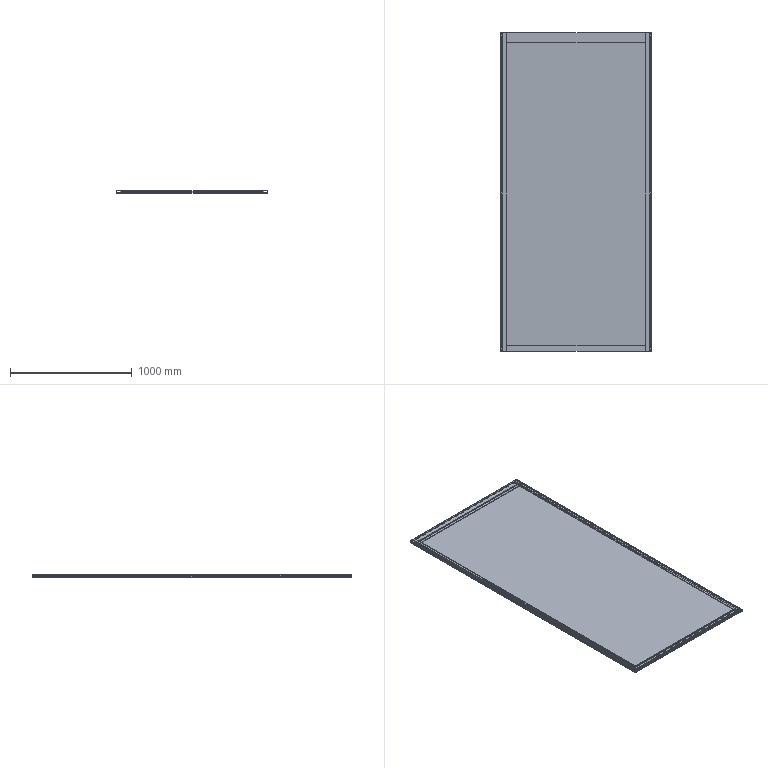Part | 5 solids | 411 faces | box 1240 x 2616 x 22 mm | volume 31479610 mm3 | plane 232 | cylinder 179 | commonest cylinder face diameters 1 x50 9 x40 0.4 x27 13 x20 14 x20 7.2 x12